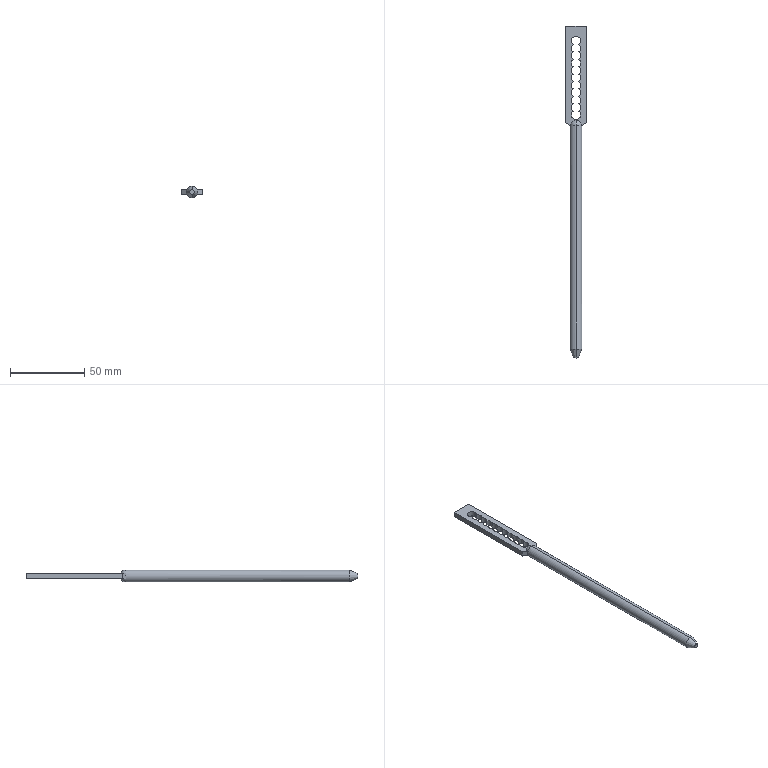Part | SolidWorks | 1 solid | 49 faces | box 14 x 224 x 8 mm | volume 10020 mm3 | cylinder 35 | plane 8 | torus 4 | cone 2 | commonest cylinder face diameters 6.1 x33 8 x2